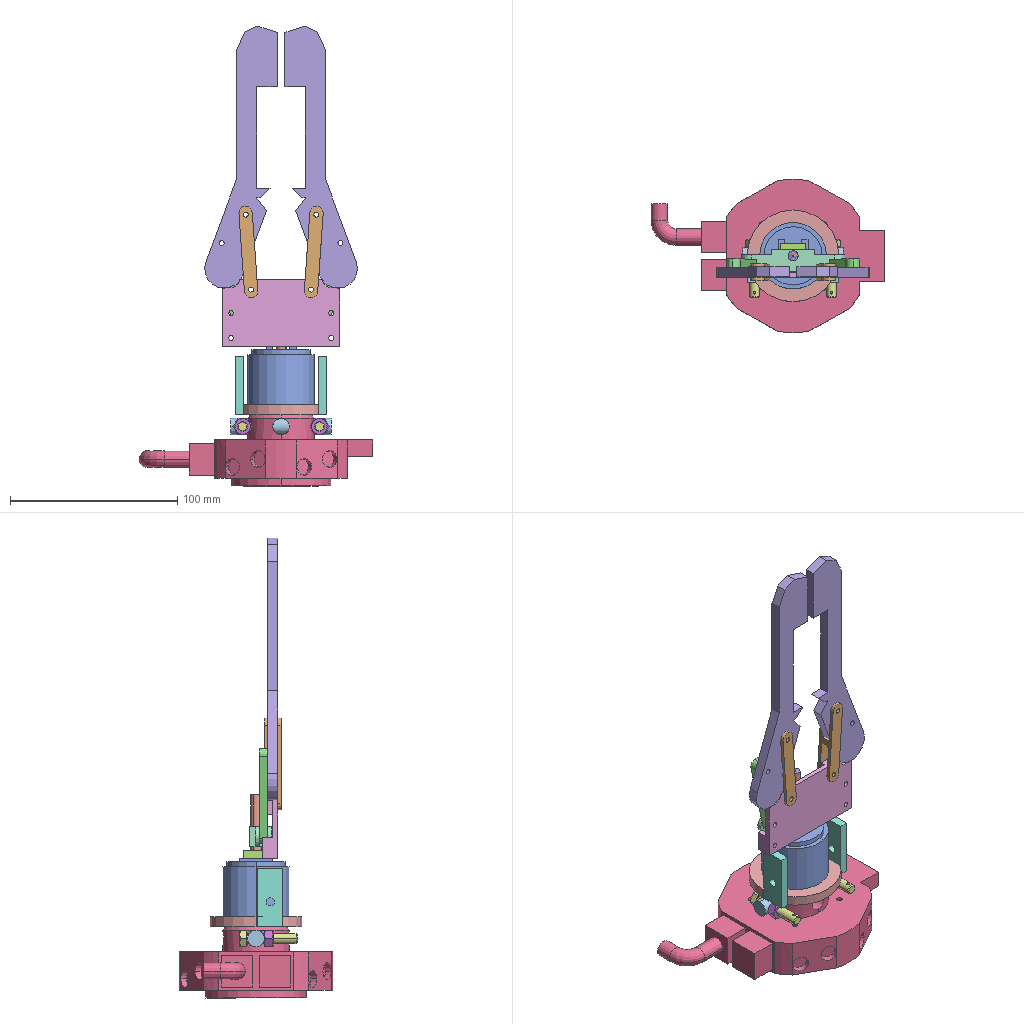Assembly | SolidWorks | 14 different items | 18 placed | box 140 x 92 x 275 mm
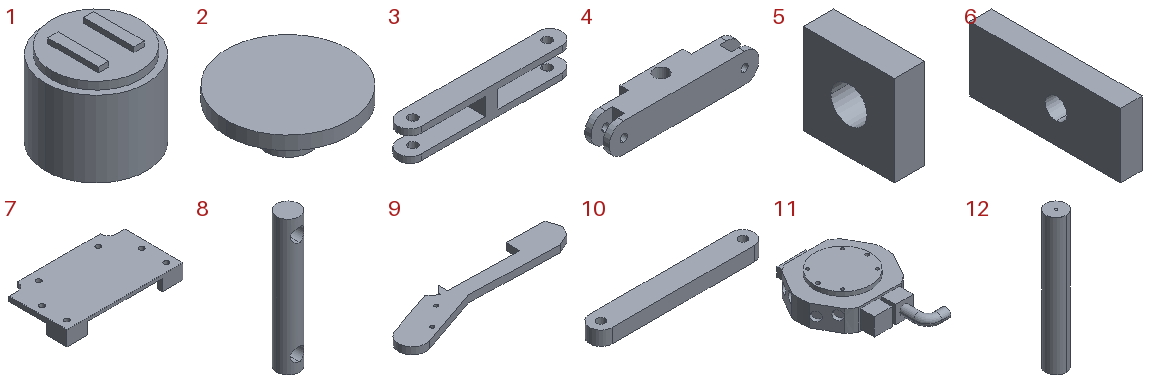Parts list (item | name | quantity | size | volume | features):
1 | - | x1 | 40 x 40 x 35 mm | 40905 mm3 | features MBimport 1
2 | - | x1 | 55 x 55 x 21 mm | 16595 mm3 | features ICE 2, CirPattern 1, MBimport 1
3 | - | x2 | 55 x 8 x 10 mm | 1841 mm3 | features MBimport 1
4 | - | x1 | 62 x 13.5 x 12 mm | 6888 mm3 | features ICE 4, Extrusion 1, MirrorSolid 1
5 | - | x1 | 5 x 15 x 15 mm | 983.628 mm3 | features MBimport 1
6 | - | x2 | 5 x 35 x 15 mm | 2527 mm3 | features MBimport 1
7 | - | x1 | 70 x 40 x 9 mm | 8600 mm3 | features MBimport 1
8 | - | x1 | 10 x 10 x 60 mm | 4174 mm3 | features Extrusion 1, ICE 1
9 | - | x2 | 157.426 x 40.732 x 6 mm | 17242 mm3 | features Chamfer 1, Extrusion 1, ICE 1
10 | - | x2 | 58 x 8 x 5 mm | 2181 mm3 | features Extrusion 1, ICE 1
11 | - | x1 | 92 x 140 x 42.6 mm | 179973 mm3 | features ICE 1, MBimport 1
12 | - | x1 | - | - | features MBimport 1
13 | hex bolts with split pin hole-grade ab gb | x1 | - | - | -
14 | hex nuts, style 1-grades ab gb | x1 | - | - | -
Mates (type | each side: item.copy, entity, surface, feature):
Concentric | 2.1 face cylinder Motor base.prt.1<1> | 1.1 face cylinder Motor.prt.1<1>
Coincident | 2.1 face plane Motor base.prt.1<1> | 1.1 face plane Motor.prt.1<1>
Coincident | 1.1 face plane Motor.prt.1<1> | 5.1 face plane Side plate.prt.1<1>
DistanceDim | 5.1 face plane Side plate.prt.1<1> | 1.1 face plane Motor.prt.1<1> | 2 times
Concentric | 5.1 face cylinder Side plate.prt.1<1> | 12.1 face cylinder Lead screw.prt.1<1>
Coincident | 1.1 face plane Motor.prt.1<1> | 12.1 face plane Lead screw.prt.1<1>
Concentric | 12.1 face cylinder Lead screw.prt.1<1> | assembly face
Concentric | assembly face | assembly face
Coincident | assembly face | assembly face
Coincident | 1.1 face plane Motor.prt.1<1> | 7.1 face plane Rear plate.prt.1<1>
Parallel | 5.1 face plane Side plate.prt.1<1> | 7.1 face plane Rear plate.prt.1<1>
DistanceDim | assembly face | 7.1 face plane Rear plate.prt.1<1>
DistanceDim | 7.1 face plane Rear plate.prt.1<1> | 5.1 face plane Side plate.prt.1<1>
Coincident | 7.1 face plane Rear plate.prt.1<1> | 6.1 face plane Side vertical plate.prt.1<1>
Parallel | 6.1 face plane Side vertical plate.prt.1<1> | assembly plane
Concentric | 7.1 edge | 3.1 edge
Coincident | 7.1 face plane Rear plate.prt.1<1> | 3.1 face plane Link.prt.1<1>
Coincident | 3.1 face plane Link.prt.1<1> | 9.1 face plane Boss-Extrude1
Concentric | 3.1 edge | 9.1 edge
Parallel | 7.1 face plane Rear plate.prt.1<1> | 9.1 face plane Boss-Extrude1
Coincident | assembly face | 10.1 face plane Boss-Extrude1
Concentric | assembly face | 10.1 edge
Concentric | 9.1 face cylinder Boss-Extrude1 | 10.1 face cylinder Cut-Extrude1
Parallel | assembly face | assembly face
LimitDistanceDim | assembly face | 12.1 face plane Lead screw.prt.1<1>
Concentric | 2.1 face cylinder Boss-Extrude1 | 11.1 face cylinder Cut-Extrude1
Coincident | 2.1 face plane Motor base.prt.1<1> | 11.1 face plane Part 16.stp<1>
Concentric | 11.1 face cylinder Part 16.stp<1> | 8.1 face cylinder Boss-Extrude1
Parallel | 2.1 face surface:4009 Cut-Extrude1 | 11.1 face cylinder Part 16.stp<1>
Parallel | 11.1 face cylinder Part 16.stp<1> | 8.1 face cylinder Cut-Extrude1
DistanceDim | 8.1 face cylinder Cut-Extrude1 | 11.1 face cylinder Part 16.stp<1>
Parallel | 8.1 face plane Boss-Extrude1 | assembly face
Perpendicular | 8.1 face cylinder Cut-Extrude1 | assembly face
DistanceDim | assembly face | 8.1 face plane Boss-Extrude1
DistanceDim | assembly face | 2.1 face plane Motor base.prt.1<1>
DistanceDim | assembly edge | 2.1 plane
Parallel | 7.1 face plane Rear plate.prt.1<1> | assembly plane
Concentric | 12.1 face cylinder Lead screw.prt.1<1> | 4.1 face cylinder Cut-Extrude2
Concentric | 10.1 face cylinder Cut-Extrude1 | 4.1 face cylinder Boss-Extrude1
Coincident | 9.1 face plane Boss-Extrude1 | 10.1 face plane Boss-Extrude1
Coincident | 10.1 face plane Boss-Extrude1 | 4.1 face plane Cut-Extrude1
LimitDistanceDim | 5.1 face plane Side plate.prt.1<1> | 4.1 face plane Boss-Extrude1